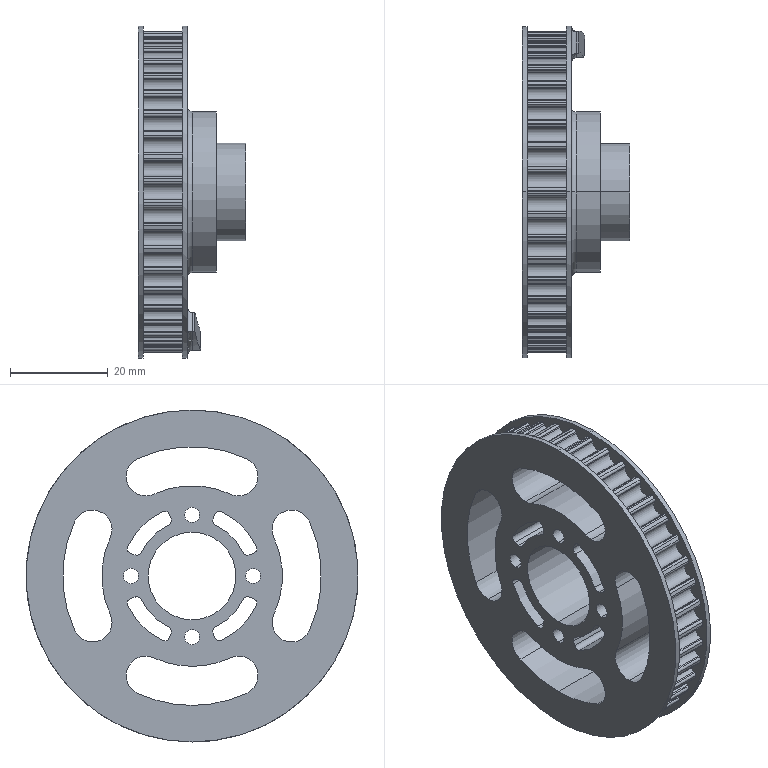Part | SolidWorks | features ICE 6, Fillet 2, BossThin 1, Chamfer 1, CirPattern 1, Cut 1, RefAxis 1, Revolution 1 | 1 solid | 395 faces | box 22 x 68 x 68 mm | volume 23228 mm3 | cylinder 285 | plane 104 | torus 6 | commonest cylinder face diameters 0.96 x104 3.12 x62 65.706 x43 2 x24 8 x12 3.1 x8